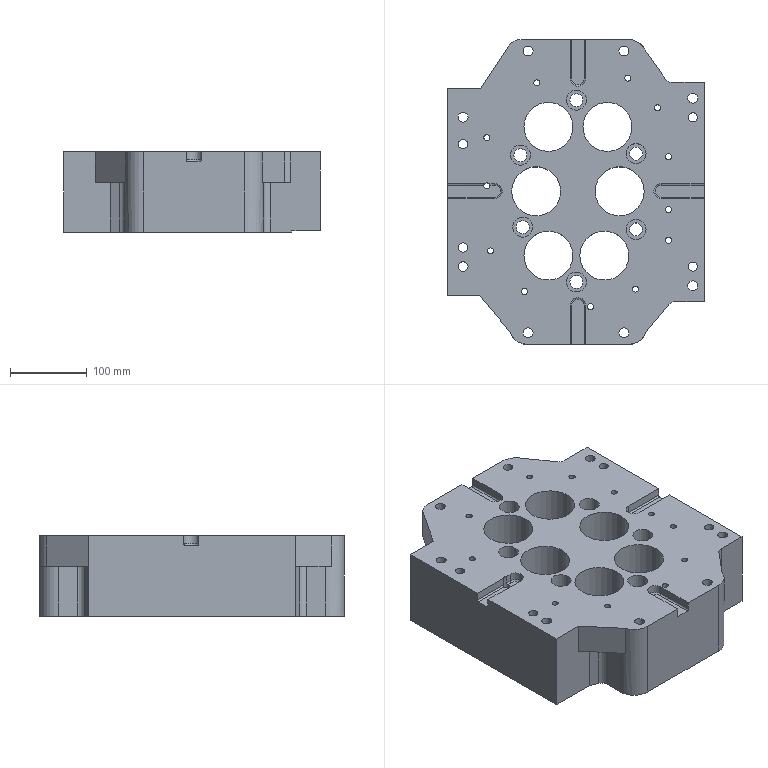Part | STEP file | 206_id1598_x_t | 1 solid | 260 faces | box 335 x 398 x 105 mm | volume 7781358 mm3 | cylinder 112 | plane 85 | cone 29 | other 24 | spline 6 | torus 4 | commonest cylinder face diameters 20 x26 6.8 x16 8 x12 13 x12 4 x9 10 x8